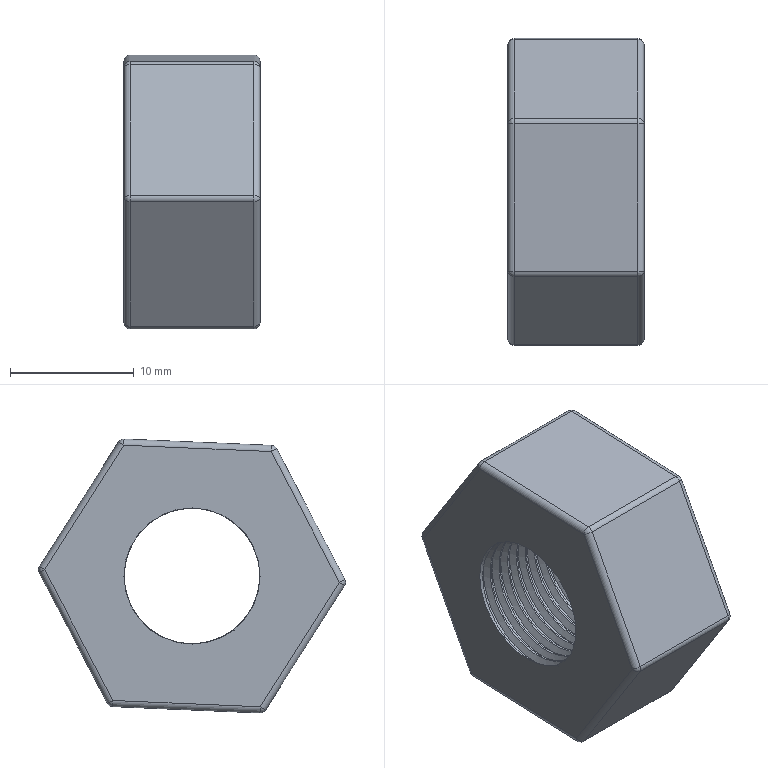Part | NX | features BLEND 2, DATUM_CSYS 2, DATUM_PLANE 1, EXTRUDE 1, SKETCH 1, THREADS 1 | 1 solid | 44 faces | box 11 x 24.824 x 22.141 mm | volume 3308 mm3 | cylinder 20 | sphere 12 | plane 10 | spline 2 | commonest cylinder face diameters 1 x18 11 x1 12 x1